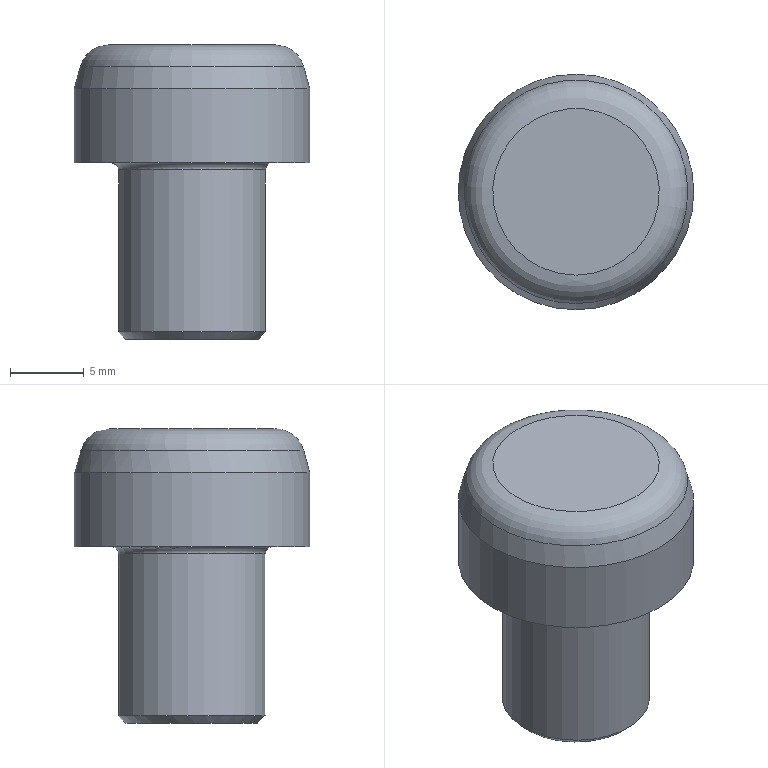Part | NX | features solid 2 | 1 solid | 9 faces | box 16 x 16 x 20 mm | volume 2471 mm3 | plane 3 | cylinder 2 | cone 2 | torus 2 | commonest cylinder face diameters 10 x1 16 x1
STEP:
#1=CARTESIAN_POINT('',(-0.000000219,-98.668,34.));
#2=VERTEX_POINT('',#1);
#3=CARTESIAN_POINT('',(-0.000000219,-93.006,34.));
#4=DIRECTION('',(0.,0.,-1.));
#5=DIRECTION('',(0.,-1.,0.));
#6=AXIS2_PLACEMENT_3D('',#3,#4,#5);
#7=CIRCLE('',#6,5.661);
#8=EDGE_CURVE('',#2,#2,#7,.T.);
#9=ORIENTED_EDGE('',*,*,#8,.F.);
#10=EDGE_LOOP('',(#9));
#11=FACE_BOUND('',#10,.T.);
#12=CARTESIAN_POINT('',(-0.000000219,-93.006,34.));
#13=DIRECTION('',(0.,0.,1.));
#14=DIRECTION('',(0.,-1.,0.));
#15=AXIS2_PLACEMENT_3D('',#12,#13,#14);
#16=PLANE('',#15);
#17=ADVANCED_FACE('',(#11),#16,.T.);
#18=CARTESIAN_POINT('',(-0.000000219,-87.506,26.));
#19=VERTEX_POINT('',#18);
#20=CARTESIAN_POINT('',(-0.000000219,-93.006,26.));
#21=DIRECTION('',(0.,0.,1.));
#22=DIRECTION('',(0.,1.,0.));
#23=AXIS2_PLACEMENT_3D('',#20,#21,#22);
#24=CIRCLE('',#23,5.5);
#25=EDGE_CURVE('',#19,#19,#24,.F.);
#26=ORIENTED_EDGE('',*,*,#25,.F.);
#27=EDGE_LOOP('',(#26));
#28=FACE_BOUND('',#27,.T.);
#29=CARTESIAN_POINT('',(-0.000000219,-101.006,26.));
#30=VERTEX_POINT('',#29);
#31=CARTESIAN_POINT('',(-0.000000219,-93.006,26.));
#32=DIRECTION('',(0.,0.,-1.));
#33=DIRECTION('',(0.,-1.,0.));
#34=AXIS2_PLACEMENT_3D('',#31,#32,#33);
#35=CIRCLE('',#34,8.);
#36=EDGE_CURVE('',#30,#30,#35,.T.);
#37=ORIENTED_EDGE('',*,*,#36,.T.);
#38=EDGE_LOOP('',(#37));
#39=FACE_BOUND('',#38,.T.);
#40=CARTESIAN_POINT('',(-0.000000219,-93.006,26.));
#41=DIRECTION('',(0.,0.,-1.));
#42=DIRECTION('',(0.,1.,0.));
#43=AXIS2_PLACEMENT_3D('',#40,#41,#42);
#44=PLANE('',#43);
#45=ADVANCED_FACE('',(#28,#39),#44,.T.);
#46=CARTESIAN_POINT('',(-0.000000219,-101.006,31.));
#47=VERTEX_POINT('',#46);
#48=CARTESIAN_POINT('',(-0.000000219,-93.006,31.));
#49=DIRECTION('',(0.,0.,-1.));
#50=DIRECTION('',(0.,-1.,0.));
#51=AXIS2_PLACEMENT_3D('',#48,#49,#50);
#52=CIRCLE('',#51,8.);
#53=EDGE_CURVE('',#47,#47,#52,.F.);
#54=ORIENTED_EDGE('',*,*,#53,.F.);
#55=EDGE_LOOP('',(#54));
#56=FACE_BOUND('',#55,.T.);
#57=ORIENTED_EDGE('',*,*,#36,.F.);
#58=EDGE_LOOP('',(#57));
#59=FACE_BOUND('',#58,.T.);
#60=CARTESIAN_POINT('',(-0.000000219,-93.006,26.));
#61=DIRECTION('',(0.,0.,1.));
#62=DIRECTION('',(0.,-1.,0.));
#63=AXIS2_PLACEMENT_3D('',#60,#61,#62);
#64=CYLINDRICAL_SURFACE('',#63,8.);
#65=ADVANCED_FACE('',(#56,#59),#64,.T.);
#66=CARTESIAN_POINT('',(-0.000000219,-100.6,32.518));
#67=VERTEX_POINT('',#66);
#68=CARTESIAN_POINT('',(-0.000000219,-93.006,32.518));
#69=DIRECTION('',(0.,0.,-1.));
#70=DIRECTION('',(0.,-1.,0.));
#71=AXIS2_PLACEMENT_3D('',#68,#69,#70);
#72=CIRCLE('',#71,7.593);
#73=EDGE_CURVE('',#67,#67,#72,.F.);
#74=ORIENTED_EDGE('',*,*,#73,.F.);
#75=EDGE_LOOP('',(#74));
#76=FACE_BOUND('',#75,.T.);
#77=ORIENTED_EDGE('',*,*,#53,.T.);
#78=EDGE_LOOP('',(#77));
#79=FACE_BOUND('',#78,.T.);
#80=CARTESIAN_POINT('',(-0.000000219,-93.006,31.));
#81=DIRECTION('',(0.,0.,-1.));
#82=DIRECTION('',(0.,1.,0.));
#83=AXIS2_PLACEMENT_3D('',#80,#81,#82);
#84=CONICAL_SURFACE('',#83,8.,0.2618);
#85=ADVANCED_FACE('',(#76,#79),#84,.T.);
#86=CARTESIAN_POINT('',(-0.000000219,-88.506,14.));
#87=VERTEX_POINT('',#86);
#88=CARTESIAN_POINT('',(-0.000000219,-93.006,14.));
#89=DIRECTION('',(0.,0.,1.));
#90=DIRECTION('',(0.,1.,0.));
#91=AXIS2_PLACEMENT_3D('',#88,#89,#90);
#92=CIRCLE('',#91,4.5);
#93=EDGE_CURVE('',#87,#87,#92,.T.);
#94=ORIENTED_EDGE('',*,*,#93,.F.);
#95=EDGE_LOOP('',(#94));
#96=FACE_BOUND('',#95,.T.);
#97=CARTESIAN_POINT('',(-0.000000219,-93.006,14.));
#98=DIRECTION('',(0.,0.,-1.));
#99=DIRECTION('',(0.,1.,0.));
#100=AXIS2_PLACEMENT_3D('',#97,#98,#99);
#101=PLANE('',#100);
#102=ADVANCED_FACE('',(#96),#101,.T.);
#103=CARTESIAN_POINT('',(-0.000000219,-88.006,25.5));
#104=VERTEX_POINT('',#103);
#105=CARTESIAN_POINT('',(-0.000000219,-93.006,25.5));
#106=DIRECTION('',(0.,0.,1.));
#107=DIRECTION('',(0.,1.,0.));
#108=AXIS2_PLACEMENT_3D('',#105,#106,#107);
#109=CIRCLE('',#108,5.);
#110=EDGE_CURVE('',#104,#104,#109,.T.);
#111=ORIENTED_EDGE('',*,*,#110,.F.);
#112=EDGE_LOOP('',(#111));
#113=FACE_BOUND('',#112,.T.);
#114=CARTESIAN_POINT('',(-0.000000219,-88.006,14.5));
#115=VERTEX_POINT('',#114);
#116=CARTESIAN_POINT('',(-0.000000219,-93.006,14.5));
#117=DIRECTION('',(0.,0.,1.));
#118=DIRECTION('',(0.,1.,0.));
#119=AXIS2_PLACEMENT_3D('',#116,#117,#118);
#120=CIRCLE('',#119,5.);
#121=EDGE_CURVE('',#115,#115,#120,.F.);
#122=ORIENTED_EDGE('',*,*,#121,.F.);
#123=EDGE_LOOP('',(#122));
#124=FACE_BOUND('',#123,.T.);
#125=CARTESIAN_POINT('',(-0.000000219,-93.006,26.));
#126=DIRECTION('',(0.,0.,-1.));
#127=DIRECTION('',(0.,1.,0.));
#128=AXIS2_PLACEMENT_3D('',#125,#126,#127);
#129=CYLINDRICAL_SURFACE('',#128,5.);
#130=ADVANCED_FACE('',(#113,#124),#129,.T.);
#131=ORIENTED_EDGE('',*,*,#93,.T.);
#132=EDGE_LOOP('',(#131));
#133=FACE_BOUND('',#132,.T.);
#134=ORIENTED_EDGE('',*,*,#121,.T.);
#135=EDGE_LOOP('',(#134));
#136=FACE_BOUND('',#135,.T.);
#137=CARTESIAN_POINT('',(-0.000000219,-93.006,14.5));
#138=DIRECTION('',(0.,0.,1.));
#139=DIRECTION('',(0.,-1.,0.));
#140=AXIS2_PLACEMENT_3D('',#137,#138,#139);
#141=CONICAL_SURFACE('',#140,5.,0.7854);
#142=ADVANCED_FACE('',(#133,#136),#141,.T.);
#143=ORIENTED_EDGE('',*,*,#25,.T.);
#144=EDGE_LOOP('',(#143));
#145=FACE_BOUND('',#144,.T.);
#146=ORIENTED_EDGE('',*,*,#110,.T.);
#147=EDGE_LOOP('',(#146));
#148=FACE_BOUND('',#147,.T.);
#149=CARTESIAN_POINT('',(-0.000000219,-93.006,25.5));
#150=DIRECTION('',(0.,0.,-1.));
#151=DIRECTION('',(0.,1.,0.));
#152=AXIS2_PLACEMENT_3D('',#149,#150,#151);
#153=TOROIDAL_SURFACE('',#152,5.5,0.5);
#154=ADVANCED_FACE('',(#145,#148),#153,.F.);
#155=ORIENTED_EDGE('',*,*,#73,.T.);
#156=EDGE_LOOP('',(#155));
#157=FACE_BOUND('',#156,.T.);
#158=ORIENTED_EDGE('',*,*,#8,.T.);
#159=EDGE_LOOP('',(#158));
#160=FACE_BOUND('',#159,.T.);
#161=CARTESIAN_POINT('',(-0.000000219,-93.006,32.));
#162=DIRECTION('',(0.,0.,1.));
#163=DIRECTION('',(0.,-1.,0.));
#164=AXIS2_PLACEMENT_3D('',#161,#162,#163);
#165=TOROIDAL_SURFACE('',#164,5.661,2.);
#166=ADVANCED_FACE('',(#157,#160),#165,.T.);
#167=CLOSED_SHELL('',(#17,#45,#65,#85,#102,#130,#142,#154,#166));
#168=MANIFOLD_SOLID_BREP('',#167);
#169=(LENGTH_UNIT()NAMED_UNIT(*)SI_UNIT(.MILLI.,.METRE.));
#170=UNCERTAINTY_MEASURE_WITH_UNIT(LENGTH_MEASURE(0.00001),#169,'','');
#171=(NAMED_UNIT(*)PLANE_ANGLE_UNIT()SI_UNIT($,.RADIAN.));
#172=(NAMED_UNIT(*)SI_UNIT($,.STERADIAN.)SOLID_ANGLE_UNIT());
#173=(GEOMETRIC_REPRESENTATION_CONTEXT(3)GLOBAL_UNCERTAINTY_ASSIGNED_CONTEXT((#170))GLOBAL_UNIT_ASSIGNED_CONTEXT((#169,#171,#172))REPRESENTATION_CONTEXT('',''));
#174=ADVANCED_BREP_SHAPE_REPRESENTATION('',(#168),#173);